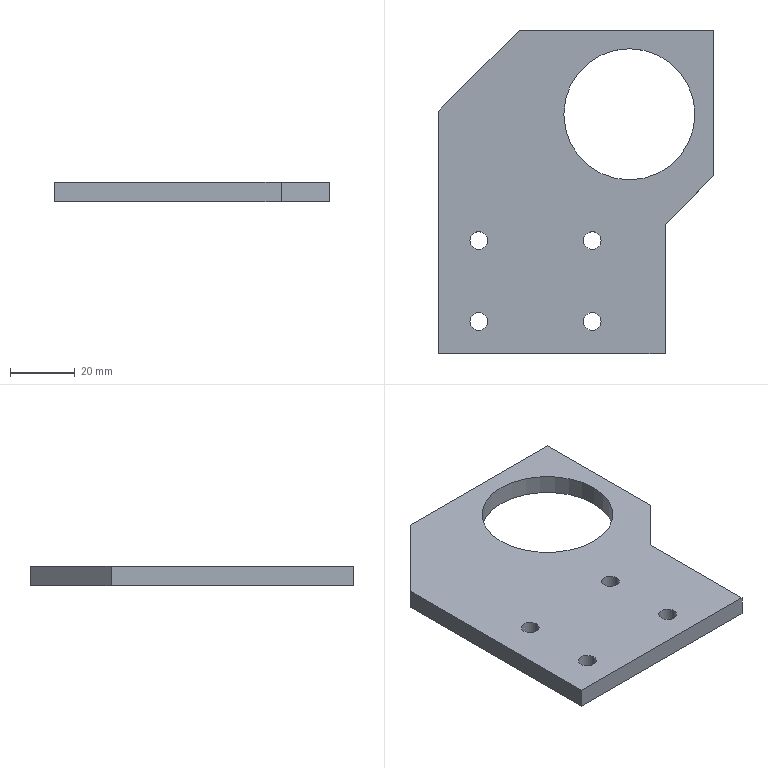Part | SolidWorks | features BaseBody 1 | 1 solid | 19 faces | box 85 x 100 x 6 mm | volume 36550 mm3 | cylinder 10 | plane 9 | commonest cylinder face diameters 5.5 x8 40.5 x2
STEP:
#1=CARTESIAN_POINT('',(-10.,100.,6.));
#2=VERTEX_POINT('',#1);
#3=CARTESIAN_POINT('',(-35.,75.,6.));
#4=VERTEX_POINT('',#3);
#5=CARTESIAN_POINT('',(-35.,75.,6.));
#6=DIRECTION('',(-0.7071,-0.7071,0.));
#7=VECTOR('',#6,1000.);
#8=LINE('',#5,#7);
#9=EDGE_CURVE('',#2,#4,#8,.T.);
#10=ORIENTED_EDGE('',*,*,#9,.F.);
#11=CARTESIAN_POINT('',(-10.,100.,0.));
#12=VERTEX_POINT('',#11);
#13=CARTESIAN_POINT('',(-10.,100.,6.));
#14=DIRECTION('',(0.,0.,1.));
#15=VECTOR('',#14,1000.);
#16=LINE('',#13,#15);
#17=EDGE_CURVE('',#12,#2,#16,.T.);
#18=ORIENTED_EDGE('',*,*,#17,.F.);
#19=CARTESIAN_POINT('',(-35.,75.,0.));
#20=VERTEX_POINT('',#19);
#21=CARTESIAN_POINT('',(-55.,55.,0.));
#22=DIRECTION('',(0.7071,0.7071,0.));
#23=VECTOR('',#22,1000.);
#24=LINE('',#21,#23);
#25=EDGE_CURVE('',#20,#12,#24,.T.);
#26=ORIENTED_EDGE('',*,*,#25,.F.);
#27=CARTESIAN_POINT('',(-35.,75.,6.));
#28=DIRECTION('',(0.,0.,-1.));
#29=VECTOR('',#28,1000.);
#30=LINE('',#27,#29);
#31=EDGE_CURVE('',#4,#20,#30,.T.);
#32=ORIENTED_EDGE('',*,*,#31,.F.);
#33=EDGE_LOOP('',(#10,#18,#26,#32));
#34=FACE_OUTER_BOUND('',#33,.T.);
#35=CARTESIAN_POINT('',(-35.,75.,6.));
#36=DIRECTION('',(0.7071,-0.7071,0.));
#37=DIRECTION('',(0.,0.,-1.));
#38=AXIS2_PLACEMENT_3D('',#35,#36,#37);
#39=PLANE('',#38);
#40=ADVANCED_FACE('',(#34),#39,.F.);
#41=CARTESIAN_POINT('',(3.749,73.999,0.));
#42=VERTEX_POINT('',#41);
#43=CARTESIAN_POINT('',(3.749,73.999,6.));
#44=VERTEX_POINT('',#43);
#45=CARTESIAN_POINT('',(3.749,73.999,0.));
#46=DIRECTION('',(0.,0.,1.));
#47=VECTOR('',#46,1000.);
#48=LINE('',#45,#47);
#49=EDGE_CURVE('',#42,#44,#48,.T.);
#50=ORIENTED_EDGE('',*,*,#49,.F.);
#51=CARTESIAN_POINT('',(44.249,73.999,0.));
#52=VERTEX_POINT('',#51);
#53=CARTESIAN_POINT('',(23.999,73.999,0.));
#54=DIRECTION('',(0.,0.,1.));
#55=DIRECTION('',(1.,0.,0.));
#56=AXIS2_PLACEMENT_3D('',#53,#54,#55);
#57=CIRCLE('',#56,20.25);
#58=EDGE_CURVE('',#52,#42,#57,.T.);
#59=ORIENTED_EDGE('',*,*,#58,.F.);
#60=CARTESIAN_POINT('',(44.249,73.999,6.));
#61=VERTEX_POINT('',#60);
#62=CARTESIAN_POINT('',(44.249,73.999,0.));
#63=DIRECTION('',(0.,0.,1.));
#64=VECTOR('',#63,1000.);
#65=LINE('',#62,#64);
#66=EDGE_CURVE('',#52,#61,#65,.T.);
#67=ORIENTED_EDGE('',*,*,#66,.T.);
#68=CARTESIAN_POINT('',(23.999,73.999,6.));
#69=DIRECTION('',(0.,0.,1.));
#70=DIRECTION('',(1.,0.,0.));
#71=AXIS2_PLACEMENT_3D('',#68,#69,#70);
#72=CIRCLE('',#71,20.25);
#73=EDGE_CURVE('',#61,#44,#72,.T.);
#74=ORIENTED_EDGE('',*,*,#73,.T.);
#75=EDGE_LOOP('',(#50,#59,#67,#74));
#76=FACE_OUTER_BOUND('',#75,.T.);
#77=CARTESIAN_POINT('',(23.999,73.999,0.));
#78=DIRECTION('',(0.,0.,1.));
#79=DIRECTION('',(1.,0.,0.));
#80=AXIS2_PLACEMENT_3D('',#77,#78,#79);
#81=CYLINDRICAL_SURFACE('',#80,20.25);
#82=ADVANCED_FACE('',(#76),#81,.F.);
#83=CARTESIAN_POINT('',(-25.25,35.,0.));
#84=VERTEX_POINT('',#83);
#85=CARTESIAN_POINT('',(-25.25,35.,6.));
#86=VERTEX_POINT('',#85);
#87=CARTESIAN_POINT('',(-25.25,35.,6.));
#88=DIRECTION('',(0.,0.,1.));
#89=VECTOR('',#88,1000.);
#90=LINE('',#87,#89);
#91=EDGE_CURVE('',#84,#86,#90,.T.);
#92=ORIENTED_EDGE('',*,*,#91,.F.);
#93=CARTESIAN_POINT('',(-19.75,35.,0.));
#94=VERTEX_POINT('',#93);
#95=CARTESIAN_POINT('',(-22.5,35.,0.));
#96=DIRECTION('',(0.,0.,1.));
#97=DIRECTION('',(1.,0.,0.));
#98=AXIS2_PLACEMENT_3D('',#95,#96,#97);
#99=CIRCLE('',#98,2.75);
#100=EDGE_CURVE('',#94,#84,#99,.T.);
#101=ORIENTED_EDGE('',*,*,#100,.F.);
#102=CARTESIAN_POINT('',(-19.75,35.,6.));
#103=VERTEX_POINT('',#102);
#104=CARTESIAN_POINT('',(-19.75,35.,6.));
#105=DIRECTION('',(0.,0.,1.));
#106=VECTOR('',#105,1000.);
#107=LINE('',#104,#106);
#108=EDGE_CURVE('',#94,#103,#107,.T.);
#109=ORIENTED_EDGE('',*,*,#108,.T.);
#110=CARTESIAN_POINT('',(-22.5,35.,6.));
#111=DIRECTION('',(0.,0.,1.));
#112=DIRECTION('',(1.,0.,0.));
#113=AXIS2_PLACEMENT_3D('',#110,#111,#112);
#114=CIRCLE('',#113,2.75);
#115=EDGE_CURVE('',#103,#86,#114,.T.);
#116=ORIENTED_EDGE('',*,*,#115,.T.);
#117=EDGE_LOOP('',(#92,#101,#109,#116));
#118=FACE_OUTER_BOUND('',#117,.T.);
#119=CARTESIAN_POINT('',(-22.5,35.,6.));
#120=DIRECTION('',(0.,0.,1.));
#121=DIRECTION('',(1.,0.,0.));
#122=AXIS2_PLACEMENT_3D('',#119,#120,#121);
#123=CYLINDRICAL_SURFACE('',#122,2.75);
#124=ADVANCED_FACE('',(#118),#123,.F.);
#125=CARTESIAN_POINT('',(-25.25,10.,0.));
#126=VERTEX_POINT('',#125);
#127=CARTESIAN_POINT('',(-25.25,10.,6.));
#128=VERTEX_POINT('',#127);
#129=CARTESIAN_POINT('',(-25.25,10.,6.));
#130=DIRECTION('',(0.,0.,1.));
#131=VECTOR('',#130,1000.);
#132=LINE('',#129,#131);
#133=EDGE_CURVE('',#126,#128,#132,.T.);
#134=ORIENTED_EDGE('',*,*,#133,.F.);
#135=CARTESIAN_POINT('',(-19.75,10.,0.));
#136=VERTEX_POINT('',#135);
#137=CARTESIAN_POINT('',(-22.5,10.,0.));
#138=DIRECTION('',(0.,0.,1.));
#139=DIRECTION('',(1.,0.,0.));
#140=AXIS2_PLACEMENT_3D('',#137,#138,#139);
#141=CIRCLE('',#140,2.75);
#142=EDGE_CURVE('',#136,#126,#141,.T.);
#143=ORIENTED_EDGE('',*,*,#142,.F.);
#144=CARTESIAN_POINT('',(-19.75,10.,6.));
#145=VERTEX_POINT('',#144);
#146=CARTESIAN_POINT('',(-19.75,10.,6.));
#147=DIRECTION('',(0.,0.,1.));
#148=VECTOR('',#147,1000.);
#149=LINE('',#146,#148);
#150=EDGE_CURVE('',#136,#145,#149,.T.);
#151=ORIENTED_EDGE('',*,*,#150,.T.);
#152=CARTESIAN_POINT('',(-22.5,10.,6.));
#153=DIRECTION('',(0.,0.,1.));
#154=DIRECTION('',(1.,0.,0.));
#155=AXIS2_PLACEMENT_3D('',#152,#153,#154);
#156=CIRCLE('',#155,2.75);
#157=EDGE_CURVE('',#145,#128,#156,.T.);
#158=ORIENTED_EDGE('',*,*,#157,.T.);
#159=EDGE_LOOP('',(#134,#143,#151,#158));
#160=FACE_OUTER_BOUND('',#159,.T.);
#161=CARTESIAN_POINT('',(-22.5,10.,6.));
#162=DIRECTION('',(0.,0.,1.));
#163=DIRECTION('',(1.,0.,0.));
#164=AXIS2_PLACEMENT_3D('',#161,#162,#163);
#165=CYLINDRICAL_SURFACE('',#164,2.75);
#166=ADVANCED_FACE('',(#160),#165,.F.);
#167=CARTESIAN_POINT('',(9.75,10.,0.));
#168=VERTEX_POINT('',#167);
#169=CARTESIAN_POINT('',(9.75,10.,6.));
#170=VERTEX_POINT('',#169);
#171=CARTESIAN_POINT('',(9.75,10.,6.));
#172=DIRECTION('',(0.,0.,1.));
#173=VECTOR('',#172,1000.);
#174=LINE('',#171,#173);
#175=EDGE_CURVE('',#168,#170,#174,.T.);
#176=ORIENTED_EDGE('',*,*,#175,.F.);
#177=CARTESIAN_POINT('',(15.25,10.,0.));
#178=VERTEX_POINT('',#177);
#179=CARTESIAN_POINT('',(12.5,10.,0.));
#180=DIRECTION('',(0.,0.,1.));
#181=DIRECTION('',(1.,0.,0.));
#182=AXIS2_PLACEMENT_3D('',#179,#180,#181);
#183=CIRCLE('',#182,2.75);
#184=EDGE_CURVE('',#178,#168,#183,.T.);
#185=ORIENTED_EDGE('',*,*,#184,.F.);
#186=CARTESIAN_POINT('',(15.25,10.,6.));
#187=VERTEX_POINT('',#186);
#188=CARTESIAN_POINT('',(15.25,10.,6.));
#189=DIRECTION('',(0.,0.,1.));
#190=VECTOR('',#189,1000.);
#191=LINE('',#188,#190);
#192=EDGE_CURVE('',#178,#187,#191,.T.);
#193=ORIENTED_EDGE('',*,*,#192,.T.);
#194=CARTESIAN_POINT('',(12.5,10.,6.));
#195=DIRECTION('',(0.,0.,1.));
#196=DIRECTION('',(1.,0.,0.));
#197=AXIS2_PLACEMENT_3D('',#194,#195,#196);
#198=CIRCLE('',#197,2.75);
#199=EDGE_CURVE('',#187,#170,#198,.T.);
#200=ORIENTED_EDGE('',*,*,#199,.T.);
#201=EDGE_LOOP('',(#176,#185,#193,#200));
#202=FACE_OUTER_BOUND('',#201,.T.);
#203=CARTESIAN_POINT('',(12.5,10.,6.));
#204=DIRECTION('',(0.,0.,1.));
#205=DIRECTION('',(1.,0.,0.));
#206=AXIS2_PLACEMENT_3D('',#203,#204,#205);
#207=CYLINDRICAL_SURFACE('',#206,2.75);
#208=ADVANCED_FACE('',(#202),#207,.F.);
#209=CARTESIAN_POINT('',(9.75,35.,0.));
#210=VERTEX_POINT('',#209);
#211=CARTESIAN_POINT('',(9.75,35.,6.));
#212=VERTEX_POINT('',#211);
#213=CARTESIAN_POINT('',(9.75,35.,6.));
#214=DIRECTION('',(0.,0.,1.));
#215=VECTOR('',#214,1000.);
#216=LINE('',#213,#215);
#217=EDGE_CURVE('',#210,#212,#216,.T.);
#218=ORIENTED_EDGE('',*,*,#217,.F.);
#219=CARTESIAN_POINT('',(15.25,35.,0.));
#220=VERTEX_POINT('',#219);
#221=CARTESIAN_POINT('',(12.5,35.,0.));
#222=DIRECTION('',(0.,0.,1.));
#223=DIRECTION('',(1.,0.,0.));
#224=AXIS2_PLACEMENT_3D('',#221,#222,#223);
#225=CIRCLE('',#224,2.75);
#226=EDGE_CURVE('',#220,#210,#225,.T.);
#227=ORIENTED_EDGE('',*,*,#226,.F.);
#228=CARTESIAN_POINT('',(15.25,35.,6.));
#229=VERTEX_POINT('',#228);
#230=CARTESIAN_POINT('',(15.25,35.,6.));
#231=DIRECTION('',(0.,0.,1.));
#232=VECTOR('',#231,1000.);
#233=LINE('',#230,#232);
#234=EDGE_CURVE('',#220,#229,#233,.T.);
#235=ORIENTED_EDGE('',*,*,#234,.T.);
#236=CARTESIAN_POINT('',(12.5,35.,6.));
#237=DIRECTION('',(0.,0.,1.));
#238=DIRECTION('',(1.,0.,0.));
#239=AXIS2_PLACEMENT_3D('',#236,#237,#238);
#240=CIRCLE('',#239,2.75);
#241=EDGE_CURVE('',#229,#212,#240,.T.);
#242=ORIENTED_EDGE('',*,*,#241,.T.);
#243=EDGE_LOOP('',(#218,#227,#235,#242));
#244=FACE_OUTER_BOUND('',#243,.T.);
#245=CARTESIAN_POINT('',(12.5,35.,6.));
#246=DIRECTION('',(0.,0.,1.));
#247=DIRECTION('',(1.,0.,0.));
#248=AXIS2_PLACEMENT_3D('',#245,#246,#247);
#249=CYLINDRICAL_SURFACE('',#248,2.75);
#250=ADVANCED_FACE('',(#244),#249,.F.);
#251=CARTESIAN_POINT('',(50.,55.,0.));
#252=VERTEX_POINT('',#251);
#253=CARTESIAN_POINT('',(50.,100.,0.));
#254=VERTEX_POINT('',#253);
#255=CARTESIAN_POINT('',(50.,100.,0.));
#256=DIRECTION('',(0.,1.,0.));
#257=VECTOR('',#256,1000.);
#258=LINE('',#255,#257);
#259=EDGE_CURVE('',#252,#254,#258,.T.);
#260=ORIENTED_EDGE('',*,*,#259,.T.);
#261=CARTESIAN_POINT('',(50.,100.,6.));
#262=VERTEX_POINT('',#261);
#263=CARTESIAN_POINT('',(50.,100.,6.));
#264=DIRECTION('',(0.,0.,-1.));
#265=VECTOR('',#264,1000.);
#266=LINE('',#263,#265);
#267=EDGE_CURVE('',#262,#254,#266,.T.);
#268=ORIENTED_EDGE('',*,*,#267,.F.);
#269=CARTESIAN_POINT('',(50.,55.,6.));
#270=VERTEX_POINT('',#269);
#271=CARTESIAN_POINT('',(50.,100.,6.));
#272=DIRECTION('',(0.,1.,0.));
#273=VECTOR('',#272,1000.);
#274=LINE('',#271,#273);
#275=EDGE_CURVE('',#270,#262,#274,.T.);
#276=ORIENTED_EDGE('',*,*,#275,.F.);
#277=CARTESIAN_POINT('',(50.,55.,6.));
#278=DIRECTION('',(0.,0.,-1.));
#279=VECTOR('',#278,1000.);
#280=LINE('',#277,#279);
#281=EDGE_CURVE('',#270,#252,#280,.T.);
#282=ORIENTED_EDGE('',*,*,#281,.T.);
#283=EDGE_LOOP('',(#260,#268,#276,#282));
#284=FACE_OUTER_BOUND('',#283,.T.);
#285=CARTESIAN_POINT('',(50.,100.,6.));
#286=DIRECTION('',(-1.,0.,0.));
#287=DIRECTION('',(0.,0.,1.));
#288=AXIS2_PLACEMENT_3D('',#285,#286,#287);
#289=PLANE('',#288);
#290=ADVANCED_FACE('',(#284),#289,.F.);
#291=CARTESIAN_POINT('',(35.,40.,0.));
#292=VERTEX_POINT('',#291);
#293=CARTESIAN_POINT('',(35.,40.,0.));
#294=DIRECTION('',(0.7071,0.7071,0.));
#295=VECTOR('',#294,1000.);
#296=LINE('',#293,#295);
#297=EDGE_CURVE('',#292,#252,#296,.T.);
#298=ORIENTED_EDGE('',*,*,#297,.T.);
#299=ORIENTED_EDGE('',*,*,#281,.F.);
#300=CARTESIAN_POINT('',(35.,40.,6.));
#301=VERTEX_POINT('',#300);
#302=CARTESIAN_POINT('',(35.,40.,6.));
#303=DIRECTION('',(0.7071,0.7071,0.));
#304=VECTOR('',#303,1000.);
#305=LINE('',#302,#304);
#306=EDGE_CURVE('',#301,#270,#305,.T.);
#307=ORIENTED_EDGE('',*,*,#306,.F.);
#308=CARTESIAN_POINT('',(35.,40.,6.));
#309=DIRECTION('',(0.,0.,-1.));
#310=VECTOR('',#309,1000.);
#311=LINE('',#308,#310);
#312=EDGE_CURVE('',#301,#292,#311,.T.);
#313=ORIENTED_EDGE('',*,*,#312,.T.);
#314=EDGE_LOOP('',(#298,#299,#307,#313));
#315=FACE_OUTER_BOUND('',#314,.T.);
#316=CARTESIAN_POINT('',(35.,40.,6.));
#317=DIRECTION('',(-0.7071,0.7071,0.));
#318=DIRECTION('',(0.,0.,1.));
#319=AXIS2_PLACEMENT_3D('',#316,#317,#318);
#320=PLANE('',#319);
#321=ADVANCED_FACE('',(#315),#320,.F.);
#322=CARTESIAN_POINT('',(35.,0.,0.));
#323=VERTEX_POINT('',#322);
#324=CARTESIAN_POINT('',(35.,0.,0.));
#325=DIRECTION('',(0.,1.,0.));
#326=VECTOR('',#325,1000.);
#327=LINE('',#324,#326);
#328=EDGE_CURVE('',#323,#292,#327,.T.);
#329=ORIENTED_EDGE('',*,*,#328,.T.);
#330=ORIENTED_EDGE('',*,*,#312,.F.);
#331=CARTESIAN_POINT('',(35.,0.,6.));
#332=VERTEX_POINT('',#331);
#333=CARTESIAN_POINT('',(35.,0.,6.));
#334=DIRECTION('',(0.,1.,0.));
#335=VECTOR('',#334,1000.);
#336=LINE('',#333,#335);
#337=EDGE_CURVE('',#332,#301,#336,.T.);
#338=ORIENTED_EDGE('',*,*,#337,.F.);
#339=CARTESIAN_POINT('',(35.,0.,6.));
#340=DIRECTION('',(0.,0.,-1.));
#341=VECTOR('',#340,1000.);
#342=LINE('',#339,#341);
#343=EDGE_CURVE('',#332,#323,#342,.T.);
#344=ORIENTED_EDGE('',*,*,#343,.T.);
#345=EDGE_LOOP('',(#329,#330,#338,#344));
#346=FACE_OUTER_BOUND('',#345,.T.);
#347=CARTESIAN_POINT('',(35.,0.,6.));
#348=DIRECTION('',(-1.,0.,0.));
#349=DIRECTION('',(0.,0.,1.));
#350=AXIS2_PLACEMENT_3D('',#347,#348,#349);
#351=PLANE('',#350);
#352=ADVANCED_FACE('',(#346),#351,.F.);
#353=CARTESIAN_POINT('',(-35.,0.,0.));
#354=VERTEX_POINT('',#353);
#355=CARTESIAN_POINT('',(-35.,0.,0.));
#356=DIRECTION('',(1.,0.,0.));
#357=VECTOR('',#356,1000.);
#358=LINE('',#355,#357);
#359=EDGE_CURVE('',#354,#323,#358,.T.);
#360=ORIENTED_EDGE('',*,*,#359,.T.);
#361=ORIENTED_EDGE('',*,*,#343,.F.);
#362=CARTESIAN_POINT('',(-35.,0.,6.));
#363=VERTEX_POINT('',#362);
#364=CARTESIAN_POINT('',(-35.,0.,6.));
#365=DIRECTION('',(1.,0.,0.));
#366=VECTOR('',#365,1000.);
#367=LINE('',#364,#366);
#368=EDGE_CURVE('',#363,#332,#367,.T.);
#369=ORIENTED_EDGE('',*,*,#368,.F.);
#370=CARTESIAN_POINT('',(-35.,0.,6.));
#371=DIRECTION('',(0.,0.,-1.));
#372=VECTOR('',#371,1000.);
#373=LINE('',#370,#372);
#374=EDGE_CURVE('',#363,#354,#373,.T.);
#375=ORIENTED_EDGE('',*,*,#374,.T.);
#376=EDGE_LOOP('',(#360,#361,#369,#375));
#377=FACE_OUTER_BOUND('',#376,.T.);
#378=CARTESIAN_POINT('',(-35.,0.,6.));
#379=DIRECTION('',(0.,1.,0.));
#380=DIRECTION('',(1.,0.,0.));
#381=AXIS2_PLACEMENT_3D('',#378,#379,#380);
#382=PLANE('',#381);
#383=ADVANCED_FACE('',(#377),#382,.F.);
#384=CARTESIAN_POINT('',(-35.,0.,6.));
#385=DIRECTION('',(0.,-1.,0.));
#386=VECTOR('',#385,1000.);
#387=LINE('',#384,#386);
#388=EDGE_CURVE('',#4,#363,#387,.T.);
#389=ORIENTED_EDGE('',*,*,#388,.F.);
#390=ORIENTED_EDGE('',*,*,#31,.T.);
#391=CARTESIAN_POINT('',(-35.,0.,0.));
#392=DIRECTION('',(0.,-1.,0.));
#393=VECTOR('',#392,1000.);
#394=LINE('',#391,#393);
#395=EDGE_CURVE('',#20,#354,#394,.T.);
#396=ORIENTED_EDGE('',*,*,#395,.T.);
#397=ORIENTED_EDGE('',*,*,#374,.F.);
#398=EDGE_LOOP('',(#389,#390,#396,#397));
#399=FACE_OUTER_BOUND('',#398,.T.);
#400=CARTESIAN_POINT('',(-35.,0.,6.));
#401=DIRECTION('',(1.,0.,0.));
#402=DIRECTION('',(0.,1.,0.));
#403=AXIS2_PLACEMENT_3D('',#400,#401,#402);
#404=PLANE('',#403);
#405=ADVANCED_FACE('',(#399),#404,.F.);
#406=CARTESIAN_POINT('',(-35.,100.,0.));
#407=DIRECTION('',(-1.,0.,0.));
#408=VECTOR('',#407,1000.);
#409=LINE('',#406,#408);
#410=EDGE_CURVE('',#254,#12,#409,.T.);
#411=ORIENTED_EDGE('',*,*,#410,.T.);
#412=ORIENTED_EDGE('',*,*,#17,.T.);
#413=CARTESIAN_POINT('',(-35.,100.,6.));
#414=DIRECTION('',(-1.,0.,0.));
#415=VECTOR('',#414,1000.);
#416=LINE('',#413,#415);
#417=EDGE_CURVE('',#262,#2,#416,.T.);
#418=ORIENTED_EDGE('',*,*,#417,.F.);
#419=ORIENTED_EDGE('',*,*,#267,.T.);
#420=EDGE_LOOP('',(#411,#412,#418,#419));
#421=FACE_OUTER_BOUND('',#420,.T.);
#422=CARTESIAN_POINT('',(-35.,100.,6.));
#423=DIRECTION('',(0.,-1.,0.));
#424=DIRECTION('',(0.,0.,-1.));
#425=AXIS2_PLACEMENT_3D('',#422,#423,#424);
#426=PLANE('',#425);
#427=ADVANCED_FACE('',(#421),#426,.F.);
#428=ORIENTED_EDGE('',*,*,#157,.F.);
#429=CARTESIAN_POINT('',(-22.5,10.,6.));
#430=DIRECTION('',(0.,0.,1.));
#431=DIRECTION('',(1.,0.,0.));
#432=AXIS2_PLACEMENT_3D('',#429,#430,#431);
#433=CIRCLE('',#432,2.75);
#434=EDGE_CURVE('',#128,#145,#433,.T.);
#435=ORIENTED_EDGE('',*,*,#434,.F.);
#436=EDGE_LOOP('',(#428,#435));
#437=FACE_BOUND('',#436,.T.);
#438=ORIENTED_EDGE('',*,*,#241,.F.);
#439=CARTESIAN_POINT('',(12.5,35.,6.));
#440=DIRECTION('',(0.,0.,1.));
#441=DIRECTION('',(1.,0.,0.));
#442=AXIS2_PLACEMENT_3D('',#439,#440,#441);
#443=CIRCLE('',#442,2.75);
#444=EDGE_CURVE('',#212,#229,#443,.T.);
#445=ORIENTED_EDGE('',*,*,#444,.F.);
#446=EDGE_LOOP('',(#438,#445));
#447=FACE_BOUND('',#446,.T.);
#448=ORIENTED_EDGE('',*,*,#199,.F.);
#449=CARTESIAN_POINT('',(12.5,10.,6.));
#450=DIRECTION('',(0.,0.,1.));
#451=DIRECTION('',(1.,0.,0.));
#452=AXIS2_PLACEMENT_3D('',#449,#450,#451);
#453=CIRCLE('',#452,2.75);
#454=EDGE_CURVE('',#170,#187,#453,.T.);
#455=ORIENTED_EDGE('',*,*,#454,.F.);
#456=EDGE_LOOP('',(#448,#455));
#457=FACE_BOUND('',#456,.T.);
#458=ORIENTED_EDGE('',*,*,#115,.F.);
#459=CARTESIAN_POINT('',(-22.5,35.,6.));
#460=DIRECTION('',(0.,0.,1.));
#461=DIRECTION('',(1.,0.,0.));
#462=AXIS2_PLACEMENT_3D('',#459,#460,#461);
#463=CIRCLE('',#462,2.75);
#464=EDGE_CURVE('',#86,#103,#463,.T.);
#465=ORIENTED_EDGE('',*,*,#464,.F.);
#466=EDGE_LOOP('',(#458,#465));
#467=FACE_BOUND('',#466,.T.);
#468=ORIENTED_EDGE('',*,*,#73,.F.);
#469=CARTESIAN_POINT('',(23.999,73.999,6.));
#470=DIRECTION('',(0.,0.,1.));
#471=DIRECTION('',(1.,0.,0.));
#472=AXIS2_PLACEMENT_3D('',#469,#470,#471);
#473=CIRCLE('',#472,20.25);
#474=EDGE_CURVE('',#44,#61,#473,.T.);
#475=ORIENTED_EDGE('',*,*,#474,.F.);
#476=EDGE_LOOP('',(#468,#475));
#477=FACE_BOUND('',#476,.T.);
#478=ORIENTED_EDGE('',*,*,#417,.T.);
#479=ORIENTED_EDGE('',*,*,#9,.T.);
#480=ORIENTED_EDGE('',*,*,#388,.T.);
#481=ORIENTED_EDGE('',*,*,#368,.T.);
#482=ORIENTED_EDGE('',*,*,#337,.T.);
#483=ORIENTED_EDGE('',*,*,#306,.T.);
#484=ORIENTED_EDGE('',*,*,#275,.T.);
#485=EDGE_LOOP('',(#478,#479,#480,#481,#482,#483,#484));
#486=FACE_OUTER_BOUND('',#485,.T.);
#487=CARTESIAN_POINT('',(0.,0.,6.));
#488=DIRECTION('',(0.,0.,-1.));
#489=DIRECTION('',(0.,-1.,0.));
#490=AXIS2_PLACEMENT_3D('',#487,#488,#489);
#491=PLANE('',#490);
#492=ADVANCED_FACE('',(#437,#447,#457,#467,#477,#486),#491,.F.);
#493=ORIENTED_EDGE('',*,*,#142,.T.);
#494=CARTESIAN_POINT('',(-22.5,10.,0.));
#495=DIRECTION('',(0.,0.,1.));
#496=DIRECTION('',(1.,0.,0.));
#497=AXIS2_PLACEMENT_3D('',#494,#495,#496);
#498=CIRCLE('',#497,2.75);
#499=EDGE_CURVE('',#126,#136,#498,.T.);
#500=ORIENTED_EDGE('',*,*,#499,.T.);
#501=EDGE_LOOP('',(#493,#500));
#502=FACE_BOUND('',#501,.T.);
#503=ORIENTED_EDGE('',*,*,#226,.T.);
#504=CARTESIAN_POINT('',(12.5,35.,0.));
#505=DIRECTION('',(0.,0.,1.));
#506=DIRECTION('',(1.,0.,0.));
#507=AXIS2_PLACEMENT_3D('',#504,#505,#506);
#508=CIRCLE('',#507,2.75);
#509=EDGE_CURVE('',#210,#220,#508,.T.);
#510=ORIENTED_EDGE('',*,*,#509,.T.);
#511=EDGE_LOOP('',(#503,#510));
#512=FACE_BOUND('',#511,.T.);
#513=ORIENTED_EDGE('',*,*,#184,.T.);
#514=CARTESIAN_POINT('',(12.5,10.,0.));
#515=DIRECTION('',(0.,0.,1.));
#516=DIRECTION('',(1.,0.,0.));
#517=AXIS2_PLACEMENT_3D('',#514,#515,#516);
#518=CIRCLE('',#517,2.75);
#519=EDGE_CURVE('',#168,#178,#518,.T.);
#520=ORIENTED_EDGE('',*,*,#519,.T.);
#521=EDGE_LOOP('',(#513,#520));
#522=FACE_BOUND('',#521,.T.);
#523=ORIENTED_EDGE('',*,*,#100,.T.);
#524=CARTESIAN_POINT('',(-22.5,35.,0.));
#525=DIRECTION('',(0.,0.,1.));
#526=DIRECTION('',(1.,0.,0.));
#527=AXIS2_PLACEMENT_3D('',#524,#525,#526);
#528=CIRCLE('',#527,2.75);
#529=EDGE_CURVE('',#84,#94,#528,.T.);
#530=ORIENTED_EDGE('',*,*,#529,.T.);
#531=EDGE_LOOP('',(#523,#530));
#532=FACE_BOUND('',#531,.T.);
#533=ORIENTED_EDGE('',*,*,#58,.T.);
#534=CARTESIAN_POINT('',(23.999,73.999,0.));
#535=DIRECTION('',(0.,0.,1.));
#536=DIRECTION('',(1.,0.,0.));
#537=AXIS2_PLACEMENT_3D('',#534,#535,#536);
#538=CIRCLE('',#537,20.25);
#539=EDGE_CURVE('',#42,#52,#538,.T.);
#540=ORIENTED_EDGE('',*,*,#539,.T.);
#541=EDGE_LOOP('',(#533,#540));
#542=FACE_BOUND('',#541,.T.);
#543=ORIENTED_EDGE('',*,*,#395,.F.);
#544=ORIENTED_EDGE('',*,*,#25,.T.);
#545=ORIENTED_EDGE('',*,*,#410,.F.);
#546=ORIENTED_EDGE('',*,*,#259,.F.);
#547=ORIENTED_EDGE('',*,*,#297,.F.);
#548=ORIENTED_EDGE('',*,*,#328,.F.);
#549=ORIENTED_EDGE('',*,*,#359,.F.);
#550=EDGE_LOOP('',(#543,#544,#545,#546,#547,#548,#549));
#551=FACE_OUTER_BOUND('',#550,.T.);
#552=CARTESIAN_POINT('',(0.,0.,0.));
#553=DIRECTION('',(0.,0.,-1.));
#554=DIRECTION('',(0.,-1.,0.));
#555=AXIS2_PLACEMENT_3D('',#552,#553,#554);
#556=PLANE('',#555);
#557=ADVANCED_FACE('',(#502,#512,#522,#532,#542,#551),#556,.T.);
#558=ORIENTED_EDGE('',*,*,#509,.F.);
#559=ORIENTED_EDGE('',*,*,#217,.T.);
#560=ORIENTED_EDGE('',*,*,#444,.T.);
#561=ORIENTED_EDGE('',*,*,#234,.F.);
#562=EDGE_LOOP('',(#558,#559,#560,#561));
#563=FACE_OUTER_BOUND('',#562,.T.);
#564=CARTESIAN_POINT('',(12.5,35.,6.));
#565=DIRECTION('',(0.,0.,1.));
#566=DIRECTION('',(1.,0.,0.));
#567=AXIS2_PLACEMENT_3D('',#564,#565,#566);
#568=CYLINDRICAL_SURFACE('',#567,2.75);
#569=ADVANCED_FACE('',(#563),#568,.F.);
#570=ORIENTED_EDGE('',*,*,#519,.F.);
#571=ORIENTED_EDGE('',*,*,#175,.T.);
#572=ORIENTED_EDGE('',*,*,#454,.T.);
#573=ORIENTED_EDGE('',*,*,#192,.F.);
#574=EDGE_LOOP('',(#570,#571,#572,#573));
#575=FACE_OUTER_BOUND('',#574,.T.);
#576=CARTESIAN_POINT('',(12.5,10.,6.));
#577=DIRECTION('',(0.,0.,1.));
#578=DIRECTION('',(1.,0.,0.));
#579=AXIS2_PLACEMENT_3D('',#576,#577,#578);
#580=CYLINDRICAL_SURFACE('',#579,2.75);
#581=ADVANCED_FACE('',(#575),#580,.F.);
#582=ORIENTED_EDGE('',*,*,#499,.F.);
#583=ORIENTED_EDGE('',*,*,#133,.T.);
#584=ORIENTED_EDGE('',*,*,#434,.T.);
#585=ORIENTED_EDGE('',*,*,#150,.F.);
#586=EDGE_LOOP('',(#582,#583,#584,#585));
#587=FACE_OUTER_BOUND('',#586,.T.);
#588=CARTESIAN_POINT('',(-22.5,10.,6.));
#589=DIRECTION('',(0.,0.,1.));
#590=DIRECTION('',(1.,0.,0.));
#591=AXIS2_PLACEMENT_3D('',#588,#589,#590);
#592=CYLINDRICAL_SURFACE('',#591,2.75);
#593=ADVANCED_FACE('',(#587),#592,.F.);
#594=ORIENTED_EDGE('',*,*,#529,.F.);
#595=ORIENTED_EDGE('',*,*,#91,.T.);
#596=ORIENTED_EDGE('',*,*,#464,.T.);
#597=ORIENTED_EDGE('',*,*,#108,.F.);
#598=EDGE_LOOP('',(#594,#595,#596,#597));
#599=FACE_OUTER_BOUND('',#598,.T.);
#600=CARTESIAN_POINT('',(-22.5,35.,6.));
#601=DIRECTION('',(0.,0.,1.));
#602=DIRECTION('',(1.,0.,0.));
#603=AXIS2_PLACEMENT_3D('',#600,#601,#602);
#604=CYLINDRICAL_SURFACE('',#603,2.75);
#605=ADVANCED_FACE('',(#599),#604,.F.);
#606=ORIENTED_EDGE('',*,*,#539,.F.);
#607=ORIENTED_EDGE('',*,*,#49,.T.);
#608=ORIENTED_EDGE('',*,*,#474,.T.);
#609=ORIENTED_EDGE('',*,*,#66,.F.);
#610=EDGE_LOOP('',(#606,#607,#608,#609));
#611=FACE_OUTER_BOUND('',#610,.T.);
#612=CARTESIAN_POINT('',(23.999,73.999,0.));
#613=DIRECTION('',(0.,0.,1.));
#614=DIRECTION('',(1.,0.,0.));
#615=AXIS2_PLACEMENT_3D('',#612,#613,#614);
#616=CYLINDRICAL_SURFACE('',#615,20.25);
#617=ADVANCED_FACE('',(#611),#616,.F.);
#618=CLOSED_SHELL('',(#40,#82,#124,#166,#208,#250,#290,#321,#352,#383,#405,#427,#492,#557,#569,#581,#593,#605,#617));
#619=MANIFOLD_SOLID_BREP('',#618);
#620=CARTESIAN_POINT('',(0.,0.,0.));
#621=DIRECTION('',(0.,0.,1.));
#622=DIRECTION('',(1.,0.,0.));
#623=AXIS2_PLACEMENT_3D('',#620,#621,#622);
#624=(LENGTH_UNIT()NAMED_UNIT(*)SI_UNIT(.MILLI.,.METRE.));
#625=UNCERTAINTY_MEASURE_WITH_UNIT(LENGTH_MEASURE(0.00001),#624,'','');
#626=(NAMED_UNIT(*)PLANE_ANGLE_UNIT()SI_UNIT($,.RADIAN.));
#627=(NAMED_UNIT(*)SI_UNIT($,.STERADIAN.)SOLID_ANGLE_UNIT());
#628=(GEOMETRIC_REPRESENTATION_CONTEXT(3)GLOBAL_UNCERTAINTY_ASSIGNED_CONTEXT((#625))GLOBAL_UNIT_ASSIGNED_CONTEXT((#624,#626,#627))REPRESENTATION_CONTEXT('',''));
#629=ADVANCED_BREP_SHAPE_REPRESENTATION('',(#619,#623),#628);